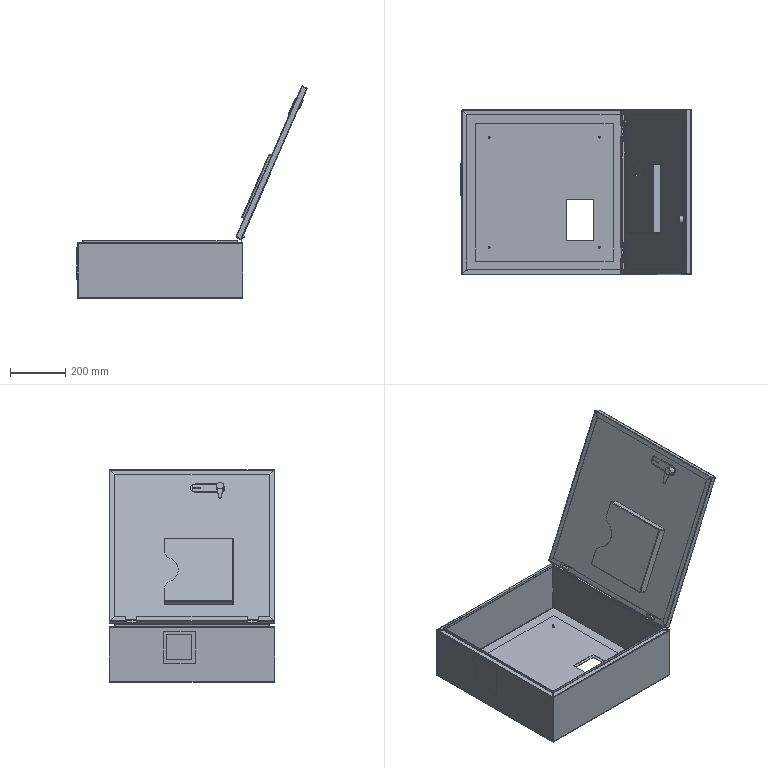Part | SolidWorks | 14 solids | 499 faces | box 837.099 x 600 x 769.432 mm | volume 2776594 mm3 | plane 332 | cylinder 131 | spline 36 | commonest cylinder face diameters 1.473 x29 4.473 x27 5 x18 7 x12 6 x10 3.3 x8